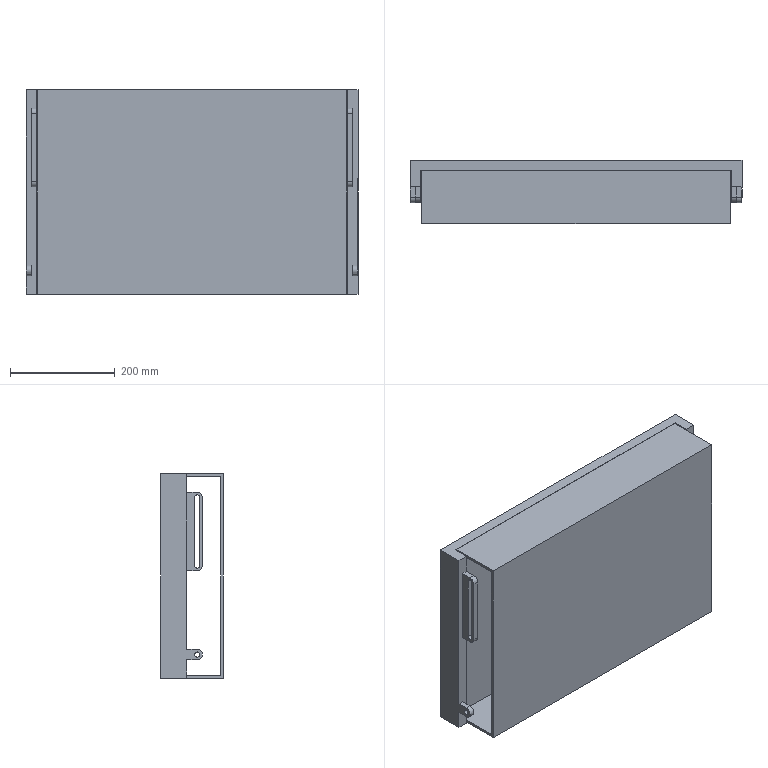Part | SolidWorks | 2 solids | 59 faces | box 634 x 120 x 390 mm | volume 7186342 mm3 | plane 43 | cylinder 16 | commonest cylinder face diameters 10 x10 20 x6